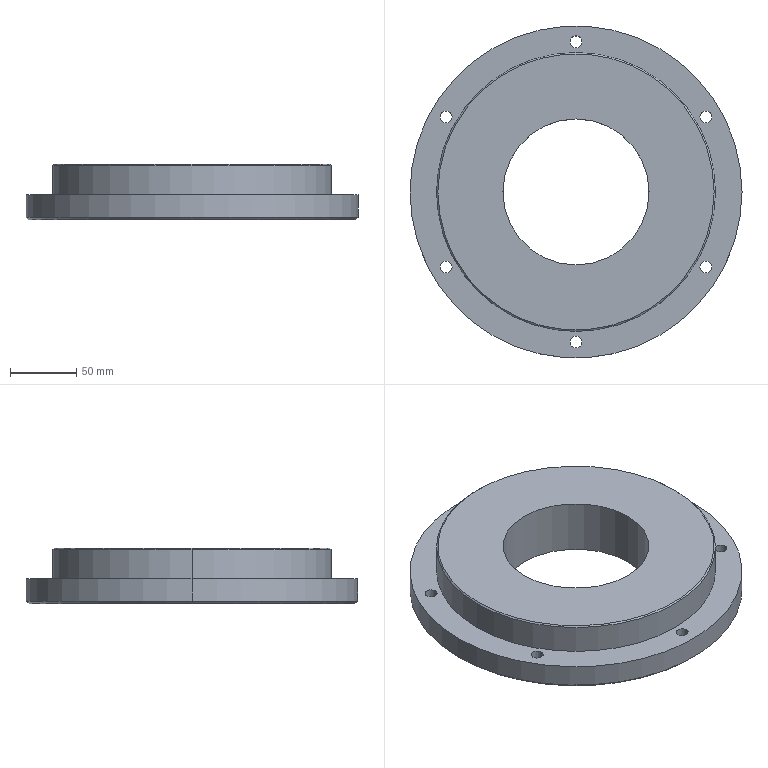Part | STEP file | Rear End Cover | 1 solid | 68 faces | box 250 x 250 x 42 mm | volume 1311495 mm3 | cylinder 44 | cone 12 | plane 12 | commonest cylinder face diameters 9 x12 16 x12 5 x8 4.5 x6 110 x2 210 x2